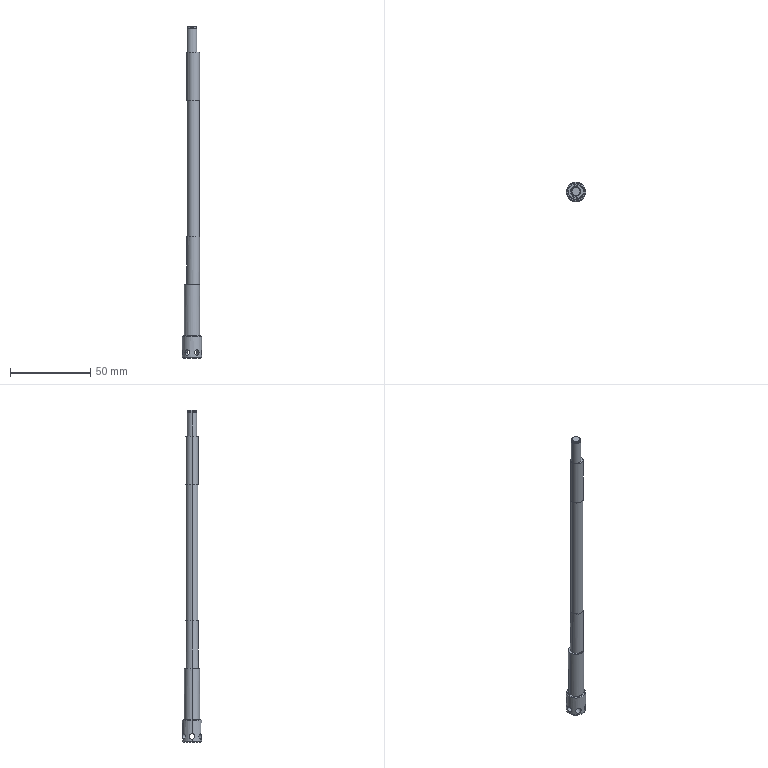Part | SolidWorks | features ICE 6, Chamfer 2, CirPattern 1, Extrusion 1, RevCut 1 | 1 solid | 43 faces | box 12 x 12 x 207.5 mm | volume 10807 mm3 | cylinder 28 | plane 9 | cone 6 | commonest cylinder face diameters 3.5 x12 6 x4 8 x4 5.6 x2 7.5 x2 9.5 x2